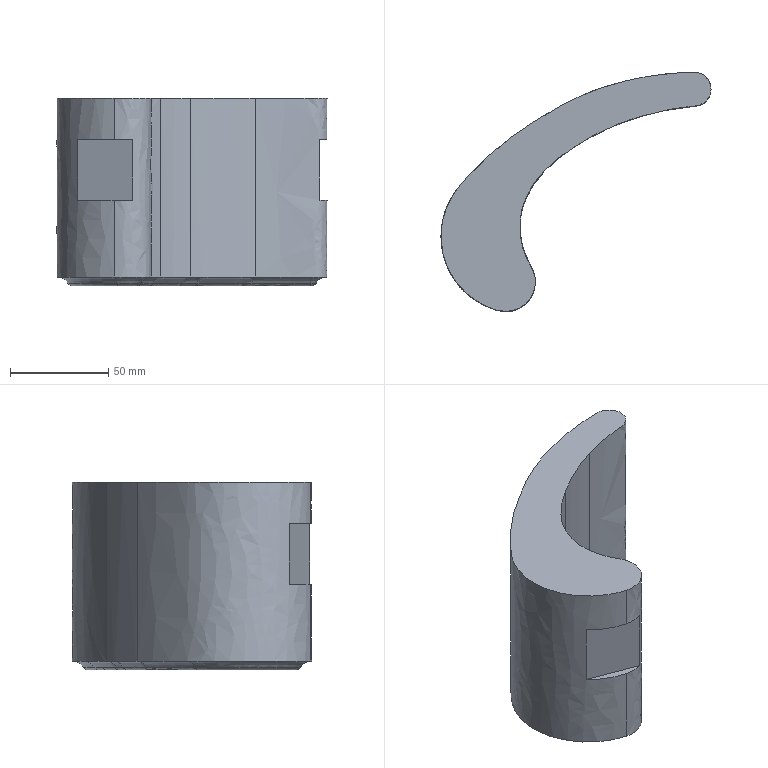Part | NX | features 8 2 | 1 solid | 42 faces | box 137.389 x 121.69 x 95.501 mm | volume 459049 mm3 | spline 18 | torus 16 | plane 8